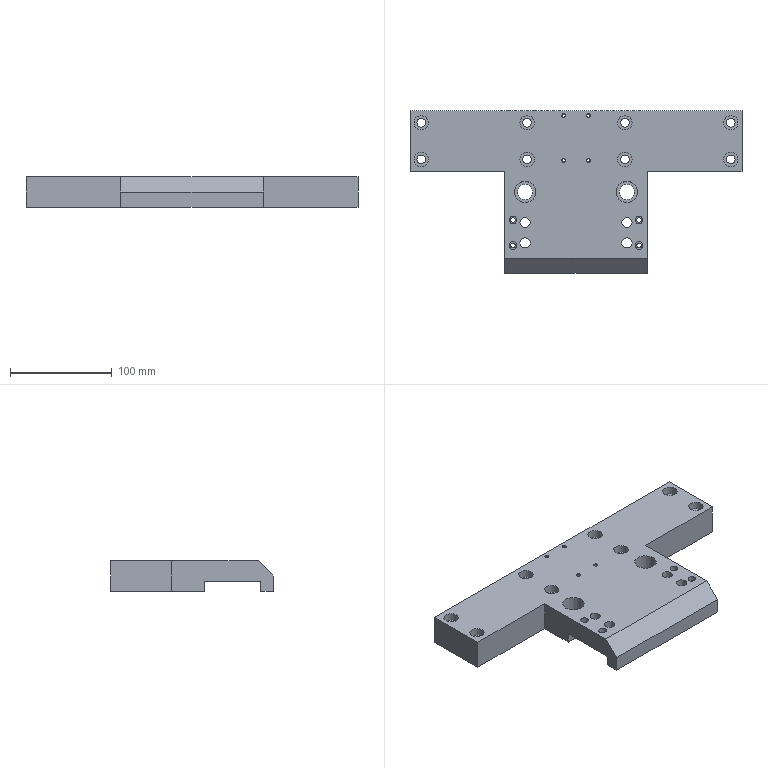Part | STEP file | Tube necking machine_id342_x_t | 1 solid | 73 faces | box 326 x 160 x 30 mm | volume 867669 mm3 | cylinder 36 | plane 29 | cone 8 | commonest cylinder face diameters 8.5 x8 14 x8 3.3 x4 4.5 x4 7.5 x4 10 x4